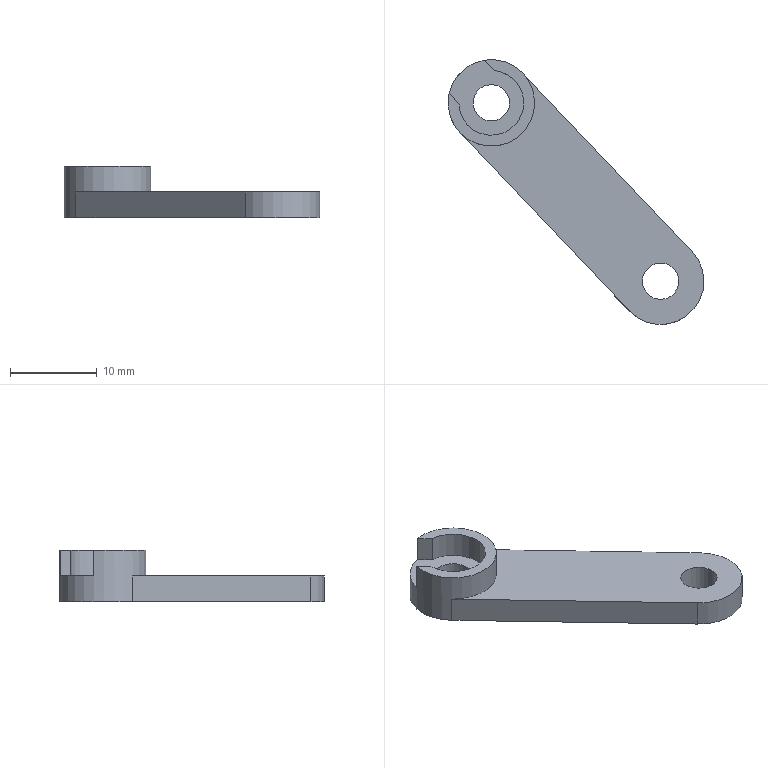Part | NX | features DATUM_CSYS 3, EXTRUDE 2, OFFSET_REGION 2, SKETCH 2, BREP 1, SCALE 1 | 1 solid | 13 faces | box 29.552 x 30.598 x 6 mm | volume 1085 mm3 | plane 8 | cylinder 5 | commonest cylinder face diameters 4.2 x2 10 x2 7.5 x1
STEP:
#1=CARTESIAN_POINT('',(-546.002,-195.798,2.5));
#2=VERTEX_POINT('',#1);
#3=CARTESIAN_POINT('',(-547.137,-194.603,2.5));
#4=VERTEX_POINT('',#3);
#5=CARTESIAN_POINT('',(-546.002,-195.798,2.5));
#6=DIRECTION('',(-0.6885,0.7253,0.));
#7=VECTOR('',#6,1000.);
#8=LINE('',#5,#7);
#9=EDGE_CURVE('',#2,#4,#8,.T.);
#10=ORIENTED_EDGE('',*,*,#9,.F.);
#11=CARTESIAN_POINT('',(-541.941,-191.943,2.5));
#12=VERTEX_POINT('',#11);
#13=CARTESIAN_POINT('',(-542.254,-195.68,2.5));
#14=DIRECTION('',(0.,0.,-1.));
#15=DIRECTION('',(0.6885,-0.7253,0.));
#16=AXIS2_PLACEMENT_3D('',#13,#14,#15);
#17=CIRCLE('',#16,3.75);
#18=EDGE_CURVE('',#12,#2,#17,.T.);
#19=ORIENTED_EDGE('',*,*,#18,.F.);
#20=CARTESIAN_POINT('',(-543.075,-190.747,2.5));
#21=VERTEX_POINT('',#20);
#22=CARTESIAN_POINT('',(-543.075,-190.747,2.5));
#23=DIRECTION('',(0.6885,-0.7253,0.));
#24=VECTOR('',#23,1000.);
#25=LINE('',#22,#24);
#26=EDGE_CURVE('',#21,#12,#25,.T.);
#27=ORIENTED_EDGE('',*,*,#26,.F.);
#28=CARTESIAN_POINT('',(-542.254,-195.68,2.5));
#29=DIRECTION('',(0.,0.,1.));
#30=DIRECTION('',(1.,0.,0.));
#31=AXIS2_PLACEMENT_3D('',#28,#29,#30);
#32=CIRCLE('',#31,5.);
#33=EDGE_CURVE('',#21,#4,#32,.T.);
#34=ORIENTED_EDGE('',*,*,#33,.T.);
#35=EDGE_LOOP('',(#10,#19,#27,#34));
#36=FACE_BOUND('',#35,.T.);
#37=CARTESIAN_POINT('',(-540.154,-195.68,2.5));
#38=VERTEX_POINT('',#37);
#39=CARTESIAN_POINT('',(-542.254,-195.68,2.5));
#40=DIRECTION('',(0.,0.,1.));
#41=DIRECTION('',(1.,0.,0.));
#42=AXIS2_PLACEMENT_3D('',#39,#40,#41);
#43=CIRCLE('',#42,2.1);
#44=EDGE_CURVE('',#38,#38,#43,.F.);
#45=ORIENTED_EDGE('',*,*,#44,.T.);
#46=EDGE_LOOP('',(#45));
#47=FACE_BOUND('',#46,.T.);
#48=CARTESIAN_POINT('',(-542.254,-195.68,2.5));
#49=DIRECTION('',(0.,0.,1.));
#50=DIRECTION('',(0.6885,-0.7253,0.));
#51=AXIS2_PLACEMENT_3D('',#48,#49,#50);
#52=PLANE('',#51);
#53=ADVANCED_FACE('',(#36,#47),#52,.T.);
#54=CARTESIAN_POINT('',(-545.88,-199.122,2.5));
#55=VERTEX_POINT('',#54);
#56=CARTESIAN_POINT('',(-545.88,-199.122,-0.5));
#57=VERTEX_POINT('',#56);
#58=CARTESIAN_POINT('',(-545.88,-199.122,0.5));
#59=DIRECTION('',(0.,0.,1.));
#60=VECTOR('',#59,1000.);
#61=LINE('',#58,#60);
#62=EDGE_CURVE('',#55,#57,#61,.F.);
#63=ORIENTED_EDGE('',*,*,#62,.F.);
#64=CARTESIAN_POINT('',(-538.628,-192.237,2.5));
#65=VERTEX_POINT('',#64);
#66=CARTESIAN_POINT('',(-542.254,-195.68,2.5));
#67=DIRECTION('',(0.,0.,1.));
#68=DIRECTION('',(0.6885,-0.7253,0.));
#69=AXIS2_PLACEMENT_3D('',#66,#67,#68);
#70=CIRCLE('',#69,5.);
#71=EDGE_CURVE('',#65,#55,#70,.F.);
#72=ORIENTED_EDGE('',*,*,#71,.F.);
#73=CARTESIAN_POINT('',(-538.628,-192.237,-0.5));
#74=VERTEX_POINT('',#73);
#75=CARTESIAN_POINT('',(-538.628,-192.237,0.5));
#76=DIRECTION('',(0.,0.,-1.));
#77=VECTOR('',#76,1000.);
#78=LINE('',#75,#77);
#79=EDGE_CURVE('',#65,#74,#78,.T.);
#80=ORIENTED_EDGE('',*,*,#79,.T.);
#81=CARTESIAN_POINT('',(-542.254,-195.68,-0.5));
#82=DIRECTION('',(0.,0.,1.));
#83=DIRECTION('',(1.,0.,0.));
#84=AXIS2_PLACEMENT_3D('',#81,#82,#83);
#85=CIRCLE('',#84,5.);
#86=EDGE_CURVE('',#74,#57,#85,.T.);
#87=ORIENTED_EDGE('',*,*,#86,.T.);
#88=EDGE_LOOP('',(#63,#72,#80,#87));
#89=FACE_BOUND('',#88,.T.);
#90=ORIENTED_EDGE('',*,*,#33,.F.);
#91=CARTESIAN_POINT('',(-543.075,-190.747,5.5));
#92=VERTEX_POINT('',#91);
#93=CARTESIAN_POINT('',(-543.075,-190.747,2.5));
#94=DIRECTION('',(0.,0.,1.));
#95=VECTOR('',#94,1000.);
#96=LINE('',#93,#95);
#97=EDGE_CURVE('',#21,#92,#96,.T.);
#98=ORIENTED_EDGE('',*,*,#97,.T.);
#99=CARTESIAN_POINT('',(-547.137,-194.603,5.5));
#100=VERTEX_POINT('',#99);
#101=CARTESIAN_POINT('',(-542.254,-195.68,5.5));
#102=DIRECTION('',(0.,0.,1.));
#103=DIRECTION('',(0.6885,-0.7253,0.));
#104=AXIS2_PLACEMENT_3D('',#101,#102,#103);
#105=CIRCLE('',#104,5.);
#106=EDGE_CURVE('',#100,#92,#105,.T.);
#107=ORIENTED_EDGE('',*,*,#106,.F.);
#108=CARTESIAN_POINT('',(-547.137,-194.603,2.5));
#109=DIRECTION('',(0.,0.,1.));
#110=VECTOR('',#109,1000.);
#111=LINE('',#108,#110);
#112=EDGE_CURVE('',#4,#100,#111,.T.);
#113=ORIENTED_EDGE('',*,*,#112,.F.);
#114=EDGE_LOOP('',(#90,#98,#107,#113));
#115=FACE_BOUND('',#114,.T.);
#116=CARTESIAN_POINT('',(-542.254,-195.68,0.5));
#117=DIRECTION('',(0.,0.,-1.));
#118=DIRECTION('',(-0.6885,0.7253,0.));
#119=AXIS2_PLACEMENT_3D('',#116,#117,#118);
#120=CYLINDRICAL_SURFACE('',#119,5.);
#121=ADVANCED_FACE('',(#89,#115),#120,.T.);
#122=CARTESIAN_POINT('',(-526.328,-219.72,-0.5));
#123=VERTEX_POINT('',#122);
#124=CARTESIAN_POINT('',(-545.88,-199.122,-0.5));
#125=DIRECTION('',(0.6885,-0.7253,0.));
#126=VECTOR('',#125,1000.);
#127=LINE('',#124,#126);
#128=EDGE_CURVE('',#57,#123,#127,.T.);
#129=ORIENTED_EDGE('',*,*,#128,.T.);
#130=CARTESIAN_POINT('',(-526.328,-219.72,2.5));
#131=VERTEX_POINT('',#130);
#132=CARTESIAN_POINT('',(-526.328,-219.72,0.5));
#133=DIRECTION('',(0.,0.,-1.));
#134=VECTOR('',#133,1000.);
#135=LINE('',#132,#134);
#136=EDGE_CURVE('',#131,#123,#135,.T.);
#137=ORIENTED_EDGE('',*,*,#136,.F.);
#138=CARTESIAN_POINT('',(-545.88,-199.122,2.5));
#139=DIRECTION('',(0.6885,-0.7253,0.));
#140=VECTOR('',#139,1000.);
#141=LINE('',#138,#140);
#142=EDGE_CURVE('',#55,#131,#141,.T.);
#143=ORIENTED_EDGE('',*,*,#142,.F.);
#144=ORIENTED_EDGE('',*,*,#62,.T.);
#145=EDGE_LOOP('',(#129,#137,#143,#144));
#146=FACE_BOUND('',#145,.T.);
#147=CARTESIAN_POINT('',(-545.88,-199.122,0.5));
#148=DIRECTION('',(0.7253,0.6885,0.));
#149=DIRECTION('',(-0.6885,0.7253,0.));
#150=AXIS2_PLACEMENT_3D('',#147,#148,#149);
#151=PLANE('',#150);
#152=ADVANCED_FACE('',(#146),#151,.F.);
#153=CARTESIAN_POINT('',(-519.075,-212.835,-0.5));
#154=VERTEX_POINT('',#153);
#155=CARTESIAN_POINT('',(-522.702,-216.277,-0.5));
#156=DIRECTION('',(0.,0.,1.));
#157=DIRECTION('',(1.,0.,0.));
#158=AXIS2_PLACEMENT_3D('',#155,#156,#157);
#159=CIRCLE('',#158,5.);
#160=EDGE_CURVE('',#123,#154,#159,.T.);
#161=ORIENTED_EDGE('',*,*,#160,.T.);
#162=CARTESIAN_POINT('',(-519.075,-212.835,2.5));
#163=VERTEX_POINT('',#162);
#164=CARTESIAN_POINT('',(-519.075,-212.835,0.5));
#165=DIRECTION('',(0.,0.,1.));
#166=VECTOR('',#165,1000.);
#167=LINE('',#164,#166);
#168=EDGE_CURVE('',#163,#154,#167,.F.);
#169=ORIENTED_EDGE('',*,*,#168,.F.);
#170=CARTESIAN_POINT('',(-522.702,-216.277,2.5));
#171=DIRECTION('',(0.,0.,1.));
#172=DIRECTION('',(1.,0.,0.));
#173=AXIS2_PLACEMENT_3D('',#170,#171,#172);
#174=CIRCLE('',#173,5.);
#175=EDGE_CURVE('',#131,#163,#174,.T.);
#176=ORIENTED_EDGE('',*,*,#175,.F.);
#177=ORIENTED_EDGE('',*,*,#136,.T.);
#178=EDGE_LOOP('',(#161,#169,#176,#177));
#179=FACE_BOUND('',#178,.T.);
#180=CARTESIAN_POINT('',(-522.702,-216.277,0.5));
#181=DIRECTION('',(0.,0.,-1.));
#182=DIRECTION('',(-0.6885,0.7253,0.));
#183=AXIS2_PLACEMENT_3D('',#180,#181,#182);
#184=CYLINDRICAL_SURFACE('',#183,5.);
#185=ADVANCED_FACE('',(#179),#184,.T.);
#186=CARTESIAN_POINT('',(-538.628,-192.237,-0.5));
#187=DIRECTION('',(-0.6885,0.7253,0.));
#188=VECTOR('',#187,1000.);
#189=LINE('',#186,#188);
#190=EDGE_CURVE('',#154,#74,#189,.T.);
#191=ORIENTED_EDGE('',*,*,#190,.T.);
#192=ORIENTED_EDGE('',*,*,#79,.F.);
#193=CARTESIAN_POINT('',(-538.628,-192.237,2.5));
#194=DIRECTION('',(-0.6885,0.7253,0.));
#195=VECTOR('',#194,1000.);
#196=LINE('',#193,#195);
#197=EDGE_CURVE('',#163,#65,#196,.T.);
#198=ORIENTED_EDGE('',*,*,#197,.F.);
#199=ORIENTED_EDGE('',*,*,#168,.T.);
#200=EDGE_LOOP('',(#191,#192,#198,#199));
#201=FACE_BOUND('',#200,.T.);
#202=CARTESIAN_POINT('',(-538.628,-192.237,0.5));
#203=DIRECTION('',(-0.7253,-0.6885,0.));
#204=DIRECTION('',(0.6885,-0.7253,0.));
#205=AXIS2_PLACEMENT_3D('',#202,#203,#204);
#206=PLANE('',#205);
#207=ADVANCED_FACE('',(#201),#206,.F.);
#208=ORIENTED_EDGE('',*,*,#71,.T.);
#209=ORIENTED_EDGE('',*,*,#142,.T.);
#210=ORIENTED_EDGE('',*,*,#175,.T.);
#211=ORIENTED_EDGE('',*,*,#197,.T.);
#212=EDGE_LOOP('',(#208,#209,#210,#211));
#213=FACE_BOUND('',#212,.T.);
#214=CARTESIAN_POINT('',(-520.602,-216.277,2.5));
#215=VERTEX_POINT('',#214);
#216=CARTESIAN_POINT('',(-522.702,-216.277,2.5));
#217=DIRECTION('',(0.,0.,1.));
#218=DIRECTION('',(1.,0.,0.));
#219=AXIS2_PLACEMENT_3D('',#216,#217,#218);
#220=CIRCLE('',#219,2.1);
#221=EDGE_CURVE('',#215,#215,#220,.F.);
#222=ORIENTED_EDGE('',*,*,#221,.T.);
#223=EDGE_LOOP('',(#222));
#224=FACE_BOUND('',#223,.T.);
#225=CARTESIAN_POINT('',(-542.254,-195.68,2.5));
#226=DIRECTION('',(0.,0.,1.));
#227=DIRECTION('',(0.6885,-0.7253,0.));
#228=AXIS2_PLACEMENT_3D('',#225,#226,#227);
#229=PLANE('',#228);
#230=ADVANCED_FACE('',(#213,#224),#229,.T.);
#231=CARTESIAN_POINT('',(-520.602,-216.277,-0.5));
#232=VERTEX_POINT('',#231);
#233=CARTESIAN_POINT('',(-522.702,-216.277,-0.5));
#234=DIRECTION('',(0.,0.,1.));
#235=DIRECTION('',(1.,0.,0.));
#236=AXIS2_PLACEMENT_3D('',#233,#234,#235);
#237=CIRCLE('',#236,2.1);
#238=EDGE_CURVE('',#232,#232,#237,.F.);
#239=ORIENTED_EDGE('',*,*,#238,.F.);
#240=EDGE_LOOP('',(#239));
#241=FACE_BOUND('',#240,.T.);
#242=CARTESIAN_POINT('',(-540.154,-195.68,-0.5));
#243=VERTEX_POINT('',#242);
#244=CARTESIAN_POINT('',(-542.254,-195.68,-0.5));
#245=DIRECTION('',(0.,0.,1.));
#246=DIRECTION('',(1.,0.,0.));
#247=AXIS2_PLACEMENT_3D('',#244,#245,#246);
#248=CIRCLE('',#247,2.1);
#249=EDGE_CURVE('',#243,#243,#248,.F.);
#250=ORIENTED_EDGE('',*,*,#249,.F.);
#251=EDGE_LOOP('',(#250));
#252=FACE_BOUND('',#251,.T.);
#253=ORIENTED_EDGE('',*,*,#86,.F.);
#254=ORIENTED_EDGE('',*,*,#190,.F.);
#255=ORIENTED_EDGE('',*,*,#160,.F.);
#256=ORIENTED_EDGE('',*,*,#128,.F.);
#257=EDGE_LOOP('',(#253,#254,#255,#256));
#258=FACE_BOUND('',#257,.T.);
#259=CARTESIAN_POINT('',(-542.254,-195.68,-0.5));
#260=DIRECTION('',(0.,0.,1.));
#261=DIRECTION('',(0.6885,-0.7253,0.));
#262=AXIS2_PLACEMENT_3D('',#259,#260,#261);
#263=PLANE('',#262);
#264=ADVANCED_FACE('',(#241,#252,#258),#263,.F.);
#265=ORIENTED_EDGE('',*,*,#44,.F.);
#266=EDGE_LOOP('',(#265));
#267=FACE_BOUND('',#266,.T.);
#268=ORIENTED_EDGE('',*,*,#249,.T.);
#269=EDGE_LOOP('',(#268));
#270=FACE_BOUND('',#269,.T.);
#271=CARTESIAN_POINT('',(-542.254,-195.68,3.5));
#272=DIRECTION('',(0.,0.,-1.));
#273=DIRECTION('',(-1.,0.,0.));
#274=AXIS2_PLACEMENT_3D('',#271,#272,#273);
#275=CYLINDRICAL_SURFACE('',#274,2.1);
#276=ADVANCED_FACE('',(#267,#270),#275,.F.);
#277=ORIENTED_EDGE('',*,*,#221,.F.);
#278=EDGE_LOOP('',(#277));
#279=FACE_BOUND('',#278,.T.);
#280=ORIENTED_EDGE('',*,*,#238,.T.);
#281=EDGE_LOOP('',(#280));
#282=FACE_BOUND('',#281,.T.);
#283=CARTESIAN_POINT('',(-522.702,-216.277,3.5));
#284=DIRECTION('',(0.,0.,-1.));
#285=DIRECTION('',(-1.,0.,0.));
#286=AXIS2_PLACEMENT_3D('',#283,#284,#285);
#287=CYLINDRICAL_SURFACE('',#286,2.1);
#288=ADVANCED_FACE('',(#279,#282),#287,.F.);
#289=CARTESIAN_POINT('',(-546.002,-195.798,5.5));
#290=VERTEX_POINT('',#289);
#291=CARTESIAN_POINT('',(-546.002,-195.798,5.5));
#292=DIRECTION('',(-0.6885,0.7253,0.));
#293=VECTOR('',#292,1000.);
#294=LINE('',#291,#293);
#295=EDGE_CURVE('',#290,#100,#294,.T.);
#296=ORIENTED_EDGE('',*,*,#295,.F.);
#297=CARTESIAN_POINT('',(-546.002,-195.798,2.5));
#298=DIRECTION('',(0.,0.,1.));
#299=VECTOR('',#298,1000.);
#300=LINE('',#297,#299);
#301=EDGE_CURVE('',#2,#290,#300,.T.);
#302=ORIENTED_EDGE('',*,*,#301,.F.);
#303=ORIENTED_EDGE('',*,*,#9,.T.);
#304=ORIENTED_EDGE('',*,*,#112,.T.);
#305=EDGE_LOOP('',(#296,#302,#303,#304));
#306=FACE_BOUND('',#305,.T.);
#307=CARTESIAN_POINT('',(-546.002,-195.798,2.5));
#308=DIRECTION('',(0.7253,0.6885,0.));
#309=DIRECTION('',(-0.6885,0.7253,0.));
#310=AXIS2_PLACEMENT_3D('',#307,#308,#309);
#311=PLANE('',#310);
#312=ADVANCED_FACE('',(#306),#311,.T.);
#313=CARTESIAN_POINT('',(-541.941,-191.943,5.5));
#314=VERTEX_POINT('',#313);
#315=CARTESIAN_POINT('',(-543.075,-190.747,5.5));
#316=DIRECTION('',(0.6885,-0.7253,0.));
#317=VECTOR('',#316,1000.);
#318=LINE('',#315,#317);
#319=EDGE_CURVE('',#92,#314,#318,.T.);
#320=ORIENTED_EDGE('',*,*,#319,.F.);
#321=ORIENTED_EDGE('',*,*,#97,.F.);
#322=ORIENTED_EDGE('',*,*,#26,.T.);
#323=CARTESIAN_POINT('',(-541.941,-191.943,2.5));
#324=DIRECTION('',(0.,0.,1.));
#325=VECTOR('',#324,1000.);
#326=LINE('',#323,#325);
#327=EDGE_CURVE('',#12,#314,#326,.T.);
#328=ORIENTED_EDGE('',*,*,#327,.T.);
#329=EDGE_LOOP('',(#320,#321,#322,#328));
#330=FACE_BOUND('',#329,.T.);
#331=CARTESIAN_POINT('',(-543.075,-190.747,2.5));
#332=DIRECTION('',(-0.7253,-0.6885,0.));
#333=DIRECTION('',(0.6885,-0.7253,0.));
#334=AXIS2_PLACEMENT_3D('',#331,#332,#333);
#335=PLANE('',#334);
#336=ADVANCED_FACE('',(#330),#335,.T.);
#337=CARTESIAN_POINT('',(-542.254,-195.68,5.5));
#338=DIRECTION('',(0.,0.,-1.));
#339=DIRECTION('',(0.6885,-0.7253,0.));
#340=AXIS2_PLACEMENT_3D('',#337,#338,#339);
#341=CIRCLE('',#340,3.75);
#342=EDGE_CURVE('',#314,#290,#341,.T.);
#343=ORIENTED_EDGE('',*,*,#342,.F.);
#344=ORIENTED_EDGE('',*,*,#327,.F.);
#345=ORIENTED_EDGE('',*,*,#18,.T.);
#346=ORIENTED_EDGE('',*,*,#301,.T.);
#347=EDGE_LOOP('',(#343,#344,#345,#346));
#348=FACE_BOUND('',#347,.T.);
#349=CARTESIAN_POINT('',(-542.254,-195.68,2.5));
#350=DIRECTION('',(0.,0.,1.));
#351=DIRECTION('',(1.,0.,0.));
#352=AXIS2_PLACEMENT_3D('',#349,#350,#351);
#353=CYLINDRICAL_SURFACE('',#352,3.75);
#354=ADVANCED_FACE('',(#348),#353,.F.);
#355=ORIENTED_EDGE('',*,*,#295,.T.);
#356=ORIENTED_EDGE('',*,*,#106,.T.);
#357=ORIENTED_EDGE('',*,*,#319,.T.);
#358=ORIENTED_EDGE('',*,*,#342,.T.);
#359=EDGE_LOOP('',(#355,#356,#357,#358));
#360=FACE_BOUND('',#359,.T.);
#361=CARTESIAN_POINT('',(-542.254,-195.68,5.5));
#362=DIRECTION('',(0.,0.,1.));
#363=DIRECTION('',(1.,0.,0.));
#364=AXIS2_PLACEMENT_3D('',#361,#362,#363);
#365=PLANE('',#364);
#366=ADVANCED_FACE('',(#360),#365,.T.);
#367=CLOSED_SHELL('',(#53,#121,#152,#185,#207,#230,#264,#276,#288,#312,#336,#354,#366));
#368=MANIFOLD_SOLID_BREP('',#367);
#369=(LENGTH_UNIT()NAMED_UNIT(*)SI_UNIT(.MILLI.,.METRE.));
#370=UNCERTAINTY_MEASURE_WITH_UNIT(LENGTH_MEASURE(0.00001),#369,'','');
#371=(NAMED_UNIT(*)PLANE_ANGLE_UNIT()SI_UNIT($,.RADIAN.));
#372=(NAMED_UNIT(*)SI_UNIT($,.STERADIAN.)SOLID_ANGLE_UNIT());
#373=(GEOMETRIC_REPRESENTATION_CONTEXT(3)GLOBAL_UNCERTAINTY_ASSIGNED_CONTEXT((#370))GLOBAL_UNIT_ASSIGNED_CONTEXT((#369,#371,#372))REPRESENTATION_CONTEXT('',''));
#374=ADVANCED_BREP_SHAPE_REPRESENTATION('',(#368),#373);